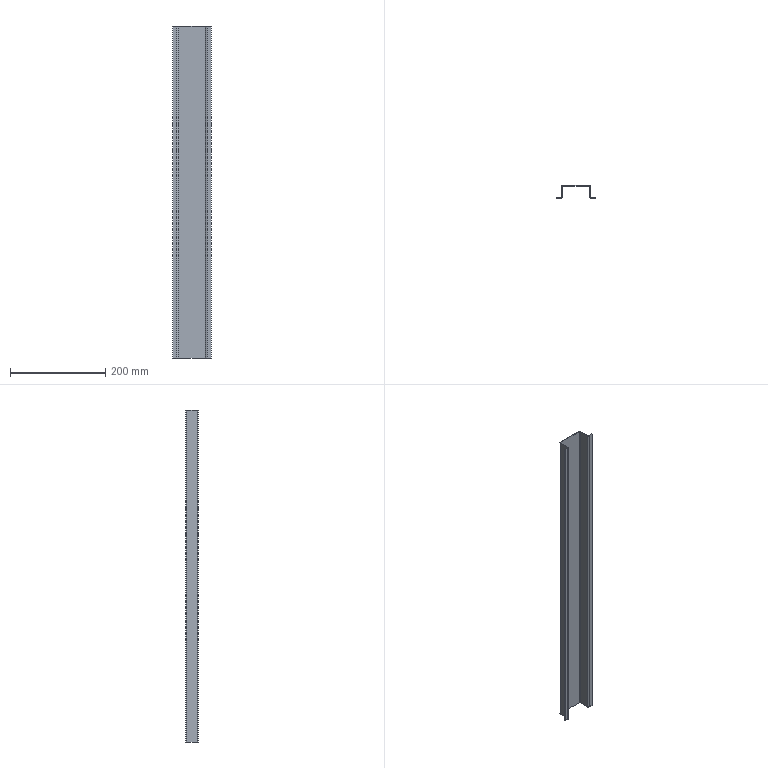Part | STEP file | Reinforcing rib | 1 solid | 22 faces | box 80 x 26.7 x 696 mm | volume 106400 mm3 | plane 14 | cylinder 8 | commonest cylinder face diameters 3 x4 5.4 x4